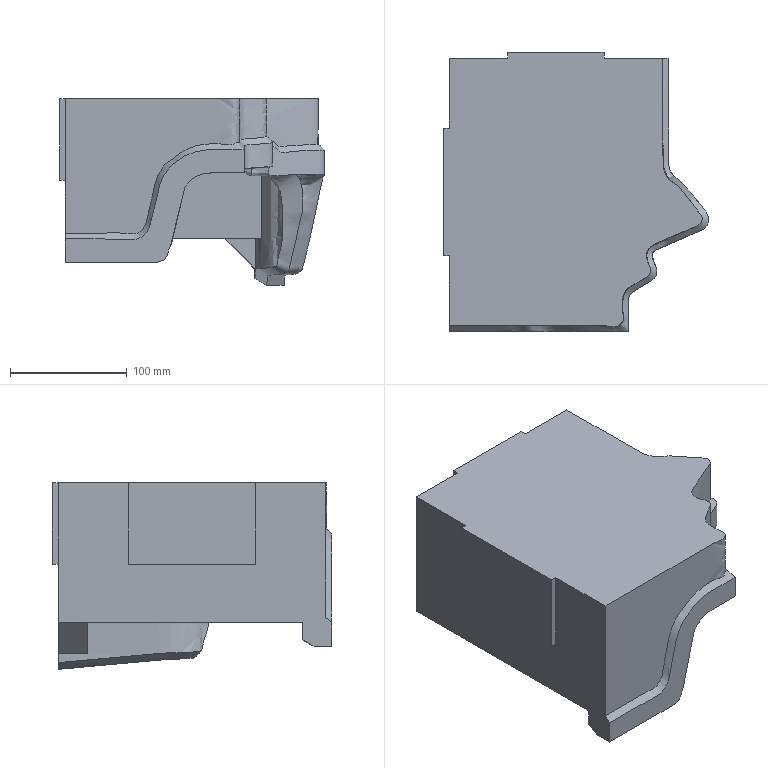Part | NX | features solid 2 | 1 solid | 40 faces | box 227.27 x 240.734 x 160.167 mm | volume 2981263 mm3 | plane 26 | spline 8 | cylinder 6 | commonest cylinder face diameters 30 x6